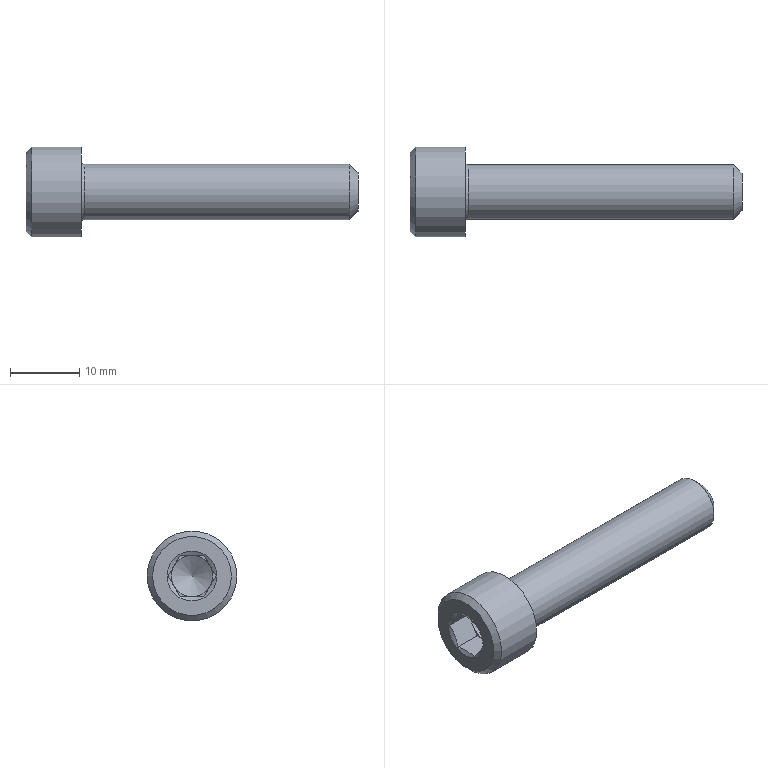Part | STEP file | Винт М8-6gx40 ГОСТ 11738-84 | 1 solid | 23 faces | box 48 x 13 x 13 mm | volume 2873 mm3 | plane 15 | cone 4 | cylinder 3 | torus 1 | commonest cylinder face diameters 6 x1 8 x1 13 x1
STEP:
#1=CARTESIAN_POINT('',(-8.,5.7,0.));
#2=VERTEX_POINT('',#1);
#3=CARTESIAN_POINT('',(-8.,0.,0.));
#4=DIRECTION('',(1.,0.,0.));
#5=DIRECTION('',(0.,1.,0.));
#6=AXIS2_PLACEMENT_3D('',#3,#4,#5);
#7=CIRCLE('',#6,5.7);
#8=EDGE_CURVE('',#2,#2,#7,.T.);
#9=ORIENTED_EDGE('',*,*,#8,.F.);
#10=EDGE_LOOP('',(#9));
#11=FACE_BOUND('',#10,.T.);
#12=CARTESIAN_POINT('',(-8.,3.6,0.));
#13=VERTEX_POINT('',#12);
#14=CARTESIAN_POINT('',(-8.,0.,0.));
#15=DIRECTION('',(1.,0.,0.));
#16=DIRECTION('',(0.,1.,0.));
#17=AXIS2_PLACEMENT_3D('',#14,#15,#16);
#18=CIRCLE('',#17,3.6);
#19=EDGE_CURVE('',#13,#13,#18,.T.);
#20=ORIENTED_EDGE('',*,*,#19,.T.);
#21=EDGE_LOOP('',(#20));
#22=FACE_BOUND('',#21,.T.);
#23=CARTESIAN_POINT('',(-8.,0.,0.));
#24=DIRECTION('',(-1.,0.,0.));
#25=DIRECTION('',(0.,1.,0.));
#26=AXIS2_PLACEMENT_3D('',#23,#24,#25);
#27=PLANE('',#26);
#28=ADVANCED_FACE('',(#11,#22),#27,.T.);
#29=CARTESIAN_POINT('',(-7.922,1.732,-3.));
#30=VERTEX_POINT('',#29);
#31=CARTESIAN_POINT('',(-7.922,-1.732,-3.));
#32=VERTEX_POINT('',#31);
#33=CARTESIAN_POINT('',(-7.922,1.732,-3.));
#34=CARTESIAN_POINT('',(-7.911,1.695,-3.));
#35=CARTESIAN_POINT('',(-7.891,1.625,-3.));
#36=CARTESIAN_POINT('',(-7.871,1.55,-3.));
#37=CARTESIAN_POINT('',(-7.851,1.474,-3.));
#38=CARTESIAN_POINT('',(-7.831,1.391,-3.));
#39=CARTESIAN_POINT('',(-7.803,1.276,-3.));
#40=CARTESIAN_POINT('',(-7.779,1.162,-3.));
#41=CARTESIAN_POINT('',(-7.76,1.068,-3.));
#42=CARTESIAN_POINT('',(-7.736,0.9374,-3.));
#43=CARTESIAN_POINT('',(-7.712,0.7953,-3.));
#44=CARTESIAN_POINT('',(-7.692,0.6398,-3.));
#45=CARTESIAN_POINT('',(-7.676,0.4906,-3.));
#46=CARTESIAN_POINT('',(-7.667,0.3765,-3.));
#47=CARTESIAN_POINT('',(-7.659,0.2523,-3.));
#48=CARTESIAN_POINT('',(-7.655,0.1456,-3.));
#49=CARTESIAN_POINT('',(-7.654,0.04767,-3.));
#50=CARTESIAN_POINT('',(-7.654,-0.05476,-3.));
#51=CARTESIAN_POINT('',(-7.655,-0.115,-3.));
#52=CARTESIAN_POINT('',(-7.658,-0.2282,-3.));
#53=CARTESIAN_POINT('',(-7.665,-0.3516,-3.));
#54=CARTESIAN_POINT('',(-7.676,-0.494,-3.));
#55=CARTESIAN_POINT('',(-7.689,-0.6078,-3.));
#56=CARTESIAN_POINT('',(-7.702,-0.7201,-3.));
#57=CARTESIAN_POINT('',(-7.719,-0.8365,-3.));
#58=CARTESIAN_POINT('',(-7.737,-0.9456,-3.));
#59=CARTESIAN_POINT('',(-7.756,-1.051,-3.));
#60=CARTESIAN_POINT('',(-7.781,-1.173,-3.));
#61=CARTESIAN_POINT('',(-7.808,-1.297,-3.));
#62=CARTESIAN_POINT('',(-7.831,-1.393,-3.));
#63=CARTESIAN_POINT('',(-7.854,-1.486,-3.));
#64=CARTESIAN_POINT('',(-7.882,-1.59,-3.));
#65=CARTESIAN_POINT('',(-7.906,-1.679,-3.));
#66=CARTESIAN_POINT('',(-7.919,-1.723,-3.));
#67=CARTESIAN_POINT('',(-7.922,-1.732,-3.));
#68=B_SPLINE_CURVE_WITH_KNOTS('',3,(#33,#34,#35,#36,#37,#38,#39,#40,#41,#42,#43,#44,#45,#46,#47,#48,#49,#50,#51,#52,#53,#54,#55,#56,#57,#58,#59,#60,#61,#62,#63,#64,#65,#66,#67),.UNSPECIFIED.,.F.,.F.,(4,1,1,1,1,1,1,1,1,1,1,1,1,1,1,1,1,1,1,1,1,1,1,1,1,1,1,1,1,1,1,1,4),(0.,0.03325,0.06137,0.06664,0.1002,0.134,0.1679,0.1994,0.2162,0.2809,0.3222,0.3499,0.4089,0.4198,0.456,0.5,0.5033,0.5434,0.5514,0.5999,0.6487,0.6732,0.6976,0.7453,0.7735,0.7919,0.8363,0.8796,0.9003,0.9208,0.9609,0.9923,1.),.UNSPECIFIED.);
#69=EDGE_CURVE('',#30,#32,#68,.T.);
#70=ORIENTED_EDGE('',*,*,#69,.T.);
#71=CARTESIAN_POINT('',(-4.,-1.732,-3.));
#72=VERTEX_POINT('',#71);
#73=CARTESIAN_POINT('',(-4.,-1.732,-3.));
#74=DIRECTION('',(-1.,0.,0.));
#75=VECTOR('',#74,1.);
#76=LINE('',#73,#75);
#77=EDGE_CURVE('',#72,#32,#76,.T.);
#78=ORIENTED_EDGE('',*,*,#77,.F.);
#79=CARTESIAN_POINT('',(-4.,0.,-3.));
#80=VERTEX_POINT('',#79);
#81=CARTESIAN_POINT('',(-4.,0.,-3.));
#82=DIRECTION('',(0.,-1.,0.));
#83=VECTOR('',#82,1.);
#84=LINE('',#81,#83);
#85=EDGE_CURVE('',#80,#72,#84,.T.);
#86=ORIENTED_EDGE('',*,*,#85,.F.);
#87=CARTESIAN_POINT('',(-4.,1.732,-3.));
#88=VERTEX_POINT('',#87);
#89=CARTESIAN_POINT('',(-4.,1.732,-3.));
#90=DIRECTION('',(0.,-1.,0.));
#91=VECTOR('',#90,1.);
#92=LINE('',#89,#91);
#93=EDGE_CURVE('',#88,#80,#92,.T.);
#94=ORIENTED_EDGE('',*,*,#93,.F.);
#95=CARTESIAN_POINT('',(-4.,1.732,-3.));
#96=DIRECTION('',(-1.,0.,0.));
#97=VECTOR('',#96,1.);
#98=LINE('',#95,#97);
#99=EDGE_CURVE('',#88,#30,#98,.T.);
#100=ORIENTED_EDGE('',*,*,#99,.T.);
#101=EDGE_LOOP('',(#70,#78,#86,#94,#100));
#102=FACE_BOUND('',#101,.T.);
#103=CARTESIAN_POINT('',(-4.,1.732,-3.));
#104=DIRECTION('',(0.,0.,-1.));
#105=DIRECTION('',(0.,-1.,0.));
#106=AXIS2_PLACEMENT_3D('',#103,#104,#105);
#107=PLANE('',#106);
#108=ADVANCED_FACE('',(#102),#107,.F.);
#109=CARTESIAN_POINT('',(-7.922,-3.464,0.));
#110=VERTEX_POINT('',#109);
#111=CARTESIAN_POINT('',(-7.922,-1.732,-3.));
#112=CARTESIAN_POINT('',(-7.911,-1.751,-2.968));
#113=CARTESIAN_POINT('',(-7.89,-1.788,-2.902));
#114=CARTESIAN_POINT('',(-7.859,-1.845,-2.804));
#115=CARTESIAN_POINT('',(-7.831,-1.902,-2.705));
#116=CARTESIAN_POINT('',(-7.803,-1.96,-2.605));
#117=CARTESIAN_POINT('',(-7.775,-2.027,-2.49));
#118=CARTESIAN_POINT('',(-7.741,-2.111,-2.343));
#119=CARTESIAN_POINT('',(-7.707,-2.216,-2.161));
#120=CARTESIAN_POINT('',(-7.68,-2.329,-1.967));
#121=CARTESIAN_POINT('',(-7.663,-2.431,-1.789));
#122=CARTESIAN_POINT('',(-7.655,-2.519,-1.637));
#123=CARTESIAN_POINT('',(-7.654,-2.574,-1.541));
#124=CARTESIAN_POINT('',(-7.654,-2.63,-1.444));
#125=CARTESIAN_POINT('',(-7.656,-2.689,-1.343));
#126=CARTESIAN_POINT('',(-7.665,-2.774,-1.196));
#127=CARTESIAN_POINT('',(-7.679,-2.859,-1.048));
#128=CARTESIAN_POINT('',(-7.698,-2.944,-0.901));
#129=CARTESIAN_POINT('',(-7.722,-3.027,-0.7571));
#130=CARTESIAN_POINT('',(-7.75,-3.107,-0.6183));
#131=CARTESIAN_POINT('',(-7.781,-3.184,-0.4844));
#132=CARTESIAN_POINT('',(-7.813,-3.258,-0.3566));
#133=CARTESIAN_POINT('',(-7.848,-3.329,-0.2336));
#134=CARTESIAN_POINT('',(-7.884,-3.397,-0.1154));
#135=CARTESIAN_POINT('',(-7.909,-3.442,-0.03806));
#136=CARTESIAN_POINT('',(-7.922,-3.464,-0.000000001));
#137=B_SPLINE_CURVE_WITH_KNOTS('',3,(#111,#112,#113,#114,#115,#116,#117,#118,#119,#120,#121,#122,#123,#124,#125,#126,#127,#128,#129,#130,#131,#132,#133,#134,#135,#136),.UNSPECIFIED.,.F.,.F.,(4,1,1,1,1,1,1,1,1,1,1,1,1,1,1,1,1,1,1,1,1,1,1,4),(0.,0.03325,0.06664,0.1002,0.134,0.1679,0.2162,0.2809,0.3499,0.4089,0.456,0.5,0.5033,0.5514,0.5999,0.6487,0.6976,0.7453,0.7919,0.8363,0.8796,0.9208,0.9609,1.),.UNSPECIFIED.);
#138=EDGE_CURVE('',#32,#110,#137,.T.);
#139=ORIENTED_EDGE('',*,*,#138,.T.);
#140=CARTESIAN_POINT('',(-4.,-3.464,0.));
#141=VERTEX_POINT('',#140);
#142=CARTESIAN_POINT('',(-4.,-3.464,0.));
#143=DIRECTION('',(-1.,0.,0.));
#144=VECTOR('',#143,1.);
#145=LINE('',#142,#144);
#146=EDGE_CURVE('',#141,#110,#145,.T.);
#147=ORIENTED_EDGE('',*,*,#146,.F.);
#148=CARTESIAN_POINT('',(-4.,-2.598,-1.5));
#149=VERTEX_POINT('',#148);
#150=CARTESIAN_POINT('',(-4.,-2.598,-1.5));
#151=DIRECTION('',(0.,-0.5,0.866));
#152=VECTOR('',#151,1.);
#153=LINE('',#150,#152);
#154=EDGE_CURVE('',#149,#141,#153,.T.);
#155=ORIENTED_EDGE('',*,*,#154,.F.);
#156=CARTESIAN_POINT('',(-4.,-1.732,-3.));
#157=DIRECTION('',(0.,-0.5,0.866));
#158=VECTOR('',#157,1.);
#159=LINE('',#156,#158);
#160=EDGE_CURVE('',#72,#149,#159,.T.);
#161=ORIENTED_EDGE('',*,*,#160,.F.);
#162=ORIENTED_EDGE('',*,*,#77,.T.);
#163=EDGE_LOOP('',(#139,#147,#155,#161,#162));
#164=FACE_BOUND('',#163,.T.);
#165=CARTESIAN_POINT('',(-4.,-1.732,-3.));
#166=DIRECTION('',(0.,-0.866,-0.5));
#167=DIRECTION('',(0.,-0.5,0.866));
#168=AXIS2_PLACEMENT_3D('',#165,#166,#167);
#169=PLANE('',#168);
#170=ADVANCED_FACE('',(#164),#169,.F.);
#171=CARTESIAN_POINT('',(-7.922,-1.732,3.));
#172=VERTEX_POINT('',#171);
#173=CARTESIAN_POINT('',(-7.922,-3.464,0.));
#174=CARTESIAN_POINT('',(-7.911,-3.445,0.03241));
#175=CARTESIAN_POINT('',(-7.89,-3.408,0.09751));
#176=CARTESIAN_POINT('',(-7.859,-3.351,0.1958));
#177=CARTESIAN_POINT('',(-7.831,-3.294,0.295));
#178=CARTESIAN_POINT('',(-7.803,-3.236,0.3951));
#179=CARTESIAN_POINT('',(-7.775,-3.17,0.5102));
#180=CARTESIAN_POINT('',(-7.741,-3.085,0.6567));
#181=CARTESIAN_POINT('',(-7.707,-2.98,0.839));
#182=CARTESIAN_POINT('',(-7.68,-2.867,1.033));
#183=CARTESIAN_POINT('',(-7.663,-2.765,1.211));
#184=CARTESIAN_POINT('',(-7.655,-2.677,1.363));
#185=CARTESIAN_POINT('',(-7.654,-2.622,1.459));
#186=CARTESIAN_POINT('',(-7.654,-2.566,1.556));
#187=CARTESIAN_POINT('',(-7.656,-2.507,1.657));
#188=CARTESIAN_POINT('',(-7.665,-2.422,1.804));
#189=CARTESIAN_POINT('',(-7.679,-2.337,1.952));
#190=CARTESIAN_POINT('',(-7.698,-2.252,2.099));
#191=CARTESIAN_POINT('',(-7.722,-2.169,2.243));
#192=CARTESIAN_POINT('',(-7.75,-2.089,2.382));
#193=CARTESIAN_POINT('',(-7.781,-2.012,2.516));
#194=CARTESIAN_POINT('',(-7.813,-1.938,2.643));
#195=CARTESIAN_POINT('',(-7.848,-1.867,2.766));
#196=CARTESIAN_POINT('',(-7.884,-1.799,2.885));
#197=CARTESIAN_POINT('',(-7.909,-1.754,2.962));
#198=CARTESIAN_POINT('',(-7.922,-1.732,3.));
#199=B_SPLINE_CURVE_WITH_KNOTS('',3,(#173,#174,#175,#176,#177,#178,#179,#180,#181,#182,#183,#184,#185,#186,#187,#188,#189,#190,#191,#192,#193,#194,#195,#196,#197,#198),.UNSPECIFIED.,.F.,.F.,(4,1,1,1,1,1,1,1,1,1,1,1,1,1,1,1,1,1,1,1,1,1,1,4),(0.,0.03325,0.06664,0.1002,0.134,0.1679,0.2162,0.2809,0.3499,0.4089,0.456,0.5,0.5033,0.5514,0.5999,0.6487,0.6976,0.7453,0.7919,0.8363,0.8796,0.9208,0.9609,1.),.UNSPECIFIED.);
#200=EDGE_CURVE('',#110,#172,#199,.T.);
#201=ORIENTED_EDGE('',*,*,#200,.T.);
#202=CARTESIAN_POINT('',(-4.,-1.732,3.));
#203=VERTEX_POINT('',#202);
#204=CARTESIAN_POINT('',(-4.,-1.732,3.));
#205=DIRECTION('',(-1.,0.,0.));
#206=VECTOR('',#205,1.);
#207=LINE('',#204,#206);
#208=EDGE_CURVE('',#203,#172,#207,.T.);
#209=ORIENTED_EDGE('',*,*,#208,.F.);
#210=CARTESIAN_POINT('',(-4.,-2.598,1.5));
#211=VERTEX_POINT('',#210);
#212=CARTESIAN_POINT('',(-4.,-2.598,1.5));
#213=DIRECTION('',(0.,0.5,0.866));
#214=VECTOR('',#213,1.);
#215=LINE('',#212,#214);
#216=EDGE_CURVE('',#211,#203,#215,.T.);
#217=ORIENTED_EDGE('',*,*,#216,.F.);
#218=CARTESIAN_POINT('',(-4.,-3.464,0.));
#219=DIRECTION('',(0.,0.5,0.866));
#220=VECTOR('',#219,1.);
#221=LINE('',#218,#220);
#222=EDGE_CURVE('',#141,#211,#221,.T.);
#223=ORIENTED_EDGE('',*,*,#222,.F.);
#224=ORIENTED_EDGE('',*,*,#146,.T.);
#225=EDGE_LOOP('',(#201,#209,#217,#223,#224));
#226=FACE_BOUND('',#225,.T.);
#227=CARTESIAN_POINT('',(-4.,-3.464,0.));
#228=DIRECTION('',(0.,-0.866,0.5));
#229=DIRECTION('',(0.,0.5,0.866));
#230=AXIS2_PLACEMENT_3D('',#227,#228,#229);
#231=PLANE('',#230);
#232=ADVANCED_FACE('',(#226),#231,.F.);
#233=CARTESIAN_POINT('',(-7.922,1.732,3.));
#234=VERTEX_POINT('',#233);
#235=CARTESIAN_POINT('',(-7.922,-1.732,3.));
#236=CARTESIAN_POINT('',(-7.911,-1.695,3.));
#237=CARTESIAN_POINT('',(-7.891,-1.625,3.));
#238=CARTESIAN_POINT('',(-7.871,-1.55,3.));
#239=CARTESIAN_POINT('',(-7.851,-1.474,3.));
#240=CARTESIAN_POINT('',(-7.831,-1.391,3.));
#241=CARTESIAN_POINT('',(-7.803,-1.276,3.));
#242=CARTESIAN_POINT('',(-7.779,-1.162,3.));
#243=CARTESIAN_POINT('',(-7.76,-1.068,3.));
#244=CARTESIAN_POINT('',(-7.736,-0.9374,3.));
#245=CARTESIAN_POINT('',(-7.712,-0.7953,3.));
#246=CARTESIAN_POINT('',(-7.692,-0.6398,3.));
#247=CARTESIAN_POINT('',(-7.676,-0.4906,3.));
#248=CARTESIAN_POINT('',(-7.667,-0.3765,3.));
#249=CARTESIAN_POINT('',(-7.659,-0.2523,3.));
#250=CARTESIAN_POINT('',(-7.655,-0.1456,3.));
#251=CARTESIAN_POINT('',(-7.654,-0.04767,3.));
#252=CARTESIAN_POINT('',(-7.654,0.05476,3.));
#253=CARTESIAN_POINT('',(-7.655,0.115,3.));
#254=CARTESIAN_POINT('',(-7.658,0.2282,3.));
#255=CARTESIAN_POINT('',(-7.665,0.3516,3.));
#256=CARTESIAN_POINT('',(-7.676,0.494,3.));
#257=CARTESIAN_POINT('',(-7.689,0.6078,3.));
#258=CARTESIAN_POINT('',(-7.702,0.7201,3.));
#259=CARTESIAN_POINT('',(-7.719,0.8365,3.));
#260=CARTESIAN_POINT('',(-7.737,0.9456,3.));
#261=CARTESIAN_POINT('',(-7.756,1.051,3.));
#262=CARTESIAN_POINT('',(-7.781,1.173,3.));
#263=CARTESIAN_POINT('',(-7.808,1.297,3.));
#264=CARTESIAN_POINT('',(-7.831,1.393,3.));
#265=CARTESIAN_POINT('',(-7.854,1.486,3.));
#266=CARTESIAN_POINT('',(-7.882,1.59,3.));
#267=CARTESIAN_POINT('',(-7.906,1.679,3.));
#268=CARTESIAN_POINT('',(-7.919,1.723,3.));
#269=CARTESIAN_POINT('',(-7.922,1.732,3.));
#270=B_SPLINE_CURVE_WITH_KNOTS('',3,(#235,#236,#237,#238,#239,#240,#241,#242,#243,#244,#245,#246,#247,#248,#249,#250,#251,#252,#253,#254,#255,#256,#257,#258,#259,#260,#261,#262,#263,#264,#265,#266,#267,#268,#269),.UNSPECIFIED.,.F.,.F.,(4,1,1,1,1,1,1,1,1,1,1,1,1,1,1,1,1,1,1,1,1,1,1,1,1,1,1,1,1,1,1,1,4),(0.,0.03325,0.06137,0.06664,0.1002,0.134,0.1679,0.1994,0.2162,0.2809,0.3222,0.3499,0.4089,0.4198,0.456,0.5,0.5033,0.5434,0.5514,0.5999,0.6487,0.6732,0.6976,0.7453,0.7735,0.7919,0.8363,0.8796,0.9003,0.9208,0.9609,0.9923,1.),.UNSPECIFIED.);
#271=EDGE_CURVE('',#172,#234,#270,.T.);
#272=ORIENTED_EDGE('',*,*,#271,.T.);
#273=CARTESIAN_POINT('',(-4.,1.732,3.));
#274=VERTEX_POINT('',#273);
#275=CARTESIAN_POINT('',(-4.,1.732,3.));
#276=DIRECTION('',(-1.,0.,0.));
#277=VECTOR('',#276,1.);
#278=LINE('',#275,#277);
#279=EDGE_CURVE('',#274,#234,#278,.T.);
#280=ORIENTED_EDGE('',*,*,#279,.F.);
#281=CARTESIAN_POINT('',(-4.,0.,3.));
#282=VERTEX_POINT('',#281);
#283=CARTESIAN_POINT('',(-4.,0.,3.));
#284=DIRECTION('',(0.,1.,0.));
#285=VECTOR('',#284,1.);
#286=LINE('',#283,#285);
#287=EDGE_CURVE('',#282,#274,#286,.T.);
#288=ORIENTED_EDGE('',*,*,#287,.F.);
#289=CARTESIAN_POINT('',(-4.,-1.732,3.));
#290=DIRECTION('',(0.,1.,0.));
#291=VECTOR('',#290,1.);
#292=LINE('',#289,#291);
#293=EDGE_CURVE('',#203,#282,#292,.T.);
#294=ORIENTED_EDGE('',*,*,#293,.F.);
#295=ORIENTED_EDGE('',*,*,#208,.T.);
#296=EDGE_LOOP('',(#272,#280,#288,#294,#295));
#297=FACE_BOUND('',#296,.T.);
#298=CARTESIAN_POINT('',(-4.,-1.732,3.));
#299=DIRECTION('',(0.,0.,1.));
#300=DIRECTION('',(0.,1.,0.));
#301=AXIS2_PLACEMENT_3D('',#298,#299,#300);
#302=PLANE('',#301);
#303=ADVANCED_FACE('',(#297),#302,.F.);
#304=CARTESIAN_POINT('',(-7.922,3.464,0.));
#305=VERTEX_POINT('',#304);
#306=CARTESIAN_POINT('',(-7.922,3.464,0.));
#307=CARTESIAN_POINT('',(-7.911,3.445,-0.03242));
#308=CARTESIAN_POINT('',(-7.89,3.408,-0.09751));
#309=CARTESIAN_POINT('',(-7.859,3.351,-0.1958));
#310=CARTESIAN_POINT('',(-7.831,3.294,-0.295));
#311=CARTESIAN_POINT('',(-7.803,3.236,-0.3951));
#312=CARTESIAN_POINT('',(-7.775,3.17,-0.5102));
#313=CARTESIAN_POINT('',(-7.741,3.085,-0.6567));
#314=CARTESIAN_POINT('',(-7.707,2.98,-0.839));
#315=CARTESIAN_POINT('',(-7.68,2.867,-1.033));
#316=CARTESIAN_POINT('',(-7.663,2.765,-1.211));
#317=CARTESIAN_POINT('',(-7.655,2.677,-1.363));
#318=CARTESIAN_POINT('',(-7.654,2.622,-1.459));
#319=CARTESIAN_POINT('',(-7.654,2.566,-1.556));
#320=CARTESIAN_POINT('',(-7.656,2.507,-1.657));
#321=CARTESIAN_POINT('',(-7.665,2.422,-1.805));
#322=CARTESIAN_POINT('',(-7.679,2.337,-1.952));
#323=CARTESIAN_POINT('',(-7.698,2.252,-2.099));
#324=CARTESIAN_POINT('',(-7.722,2.169,-2.243));
#325=CARTESIAN_POINT('',(-7.75,2.089,-2.382));
#326=CARTESIAN_POINT('',(-7.781,2.012,-2.516));
#327=CARTESIAN_POINT('',(-7.813,1.938,-2.643));
#328=CARTESIAN_POINT('',(-7.848,1.867,-2.766));
#329=CARTESIAN_POINT('',(-7.884,1.799,-2.885));
#330=CARTESIAN_POINT('',(-7.909,1.754,-2.962));
#331=CARTESIAN_POINT('',(-7.922,1.732,-3.));
#332=B_SPLINE_CURVE_WITH_KNOTS('',3,(#306,#307,#308,#309,#310,#311,#312,#313,#314,#315,#316,#317,#318,#319,#320,#321,#322,#323,#324,#325,#326,#327,#328,#329,#330,#331),.UNSPECIFIED.,.F.,.F.,(4,1,1,1,1,1,1,1,1,1,1,1,1,1,1,1,1,1,1,1,1,1,1,4),(0.,0.03325,0.06664,0.1002,0.134,0.1679,0.2162,0.2809,0.3499,0.4089,0.456,0.5,0.5033,0.5514,0.5999,0.6487,0.6976,0.7453,0.7919,0.8363,0.8796,0.9208,0.9609,1.),.UNSPECIFIED.);
#333=EDGE_CURVE('',#305,#30,#332,.T.);
#334=ORIENTED_EDGE('',*,*,#333,.T.);
#335=ORIENTED_EDGE('',*,*,#99,.F.);
#336=CARTESIAN_POINT('',(-4.,2.598,-1.5));
#337=VERTEX_POINT('',#336);
#338=CARTESIAN_POINT('',(-4.,2.598,-1.5));
#339=DIRECTION('',(0.,-0.5,-0.866));
#340=VECTOR('',#339,1.);
#341=LINE('',#338,#340);
#342=EDGE_CURVE('',#337,#88,#341,.T.);
#343=ORIENTED_EDGE('',*,*,#342,.F.);
#344=CARTESIAN_POINT('',(-4.,3.464,0.));
#345=VERTEX_POINT('',#344);
#346=CARTESIAN_POINT('',(-4.,3.464,0.));
#347=DIRECTION('',(0.,-0.5,-0.866));
#348=VECTOR('',#347,1.);
#349=LINE('',#346,#348);
#350=EDGE_CURVE('',#345,#337,#349,.T.);
#351=ORIENTED_EDGE('',*,*,#350,.F.);
#352=CARTESIAN_POINT('',(-4.,3.464,0.));
#353=DIRECTION('',(-1.,0.,0.));
#354=VECTOR('',#353,1.);
#355=LINE('',#352,#354);
#356=EDGE_CURVE('',#345,#305,#355,.T.);
#357=ORIENTED_EDGE('',*,*,#356,.T.);
#358=EDGE_LOOP('',(#334,#335,#343,#351,#357));
#359=FACE_BOUND('',#358,.T.);
#360=CARTESIAN_POINT('',(-4.,3.464,0.));
#361=DIRECTION('',(0.,0.866,-0.5));
#362=DIRECTION('',(0.,-0.5,-0.866));
#363=AXIS2_PLACEMENT_3D('',#360,#361,#362);
#364=PLANE('',#363);
#365=ADVANCED_FACE('',(#359),#364,.F.);
#366=CARTESIAN_POINT('',(-7.922,1.732,3.));
#367=CARTESIAN_POINT('',(-7.911,1.751,2.968));
#368=CARTESIAN_POINT('',(-7.89,1.788,2.902));
#369=CARTESIAN_POINT('',(-7.859,1.845,2.804));
#370=CARTESIAN_POINT('',(-7.831,1.902,2.705));
#371=CARTESIAN_POINT('',(-7.803,1.96,2.605));
#372=CARTESIAN_POINT('',(-7.775,2.027,2.49));
#373=CARTESIAN_POINT('',(-7.741,2.111,2.343));
#374=CARTESIAN_POINT('',(-7.707,2.216,2.161));
#375=CARTESIAN_POINT('',(-7.68,2.329,1.967));
#376=CARTESIAN_POINT('',(-7.663,2.431,1.789));
#377=CARTESIAN_POINT('',(-7.655,2.519,1.637));
#378=CARTESIAN_POINT('',(-7.654,2.574,1.541));
#379=CARTESIAN_POINT('',(-7.654,2.63,1.444));
#380=CARTESIAN_POINT('',(-7.656,2.689,1.343));
#381=CARTESIAN_POINT('',(-7.665,2.774,1.195));
#382=CARTESIAN_POINT('',(-7.679,2.859,1.048));
#383=CARTESIAN_POINT('',(-7.698,2.944,0.9009));
#384=CARTESIAN_POINT('',(-7.722,3.027,0.7571));
#385=CARTESIAN_POINT('',(-7.75,3.107,0.6183));
#386=CARTESIAN_POINT('',(-7.781,3.184,0.4844));
#387=CARTESIAN_POINT('',(-7.813,3.258,0.3566));
#388=CARTESIAN_POINT('',(-7.848,3.329,0.2336));
#389=CARTESIAN_POINT('',(-7.884,3.397,0.1154));
#390=CARTESIAN_POINT('',(-7.909,3.442,0.03806));
#391=CARTESIAN_POINT('',(-7.922,3.464,0.));
#392=B_SPLINE_CURVE_WITH_KNOTS('',3,(#366,#367,#368,#369,#370,#371,#372,#373,#374,#375,#376,#377,#378,#379,#380,#381,#382,#383,#384,#385,#386,#387,#388,#389,#390,#391),.UNSPECIFIED.,.F.,.F.,(4,1,1,1,1,1,1,1,1,1,1,1,1,1,1,1,1,1,1,1,1,1,1,4),(0.,0.03325,0.06664,0.1002,0.134,0.1679,0.2162,0.2809,0.3499,0.4089,0.456,0.5,0.5033,0.5514,0.5999,0.6487,0.6976,0.7453,0.7919,0.8363,0.8796,0.9208,0.9609,1.),.UNSPECIFIED.);
#393=EDGE_CURVE('',#234,#305,#392,.T.);
#394=ORIENTED_EDGE('',*,*,#393,.T.);
#395=ORIENTED_EDGE('',*,*,#356,.F.);
#396=CARTESIAN_POINT('',(-4.,2.598,1.5));
#397=VERTEX_POINT('',#396);
#398=CARTESIAN_POINT('',(-4.,2.598,1.5));
#399=DIRECTION('',(0.,0.5,-0.866));
#400=VECTOR('',#399,1.);
#401=LINE('',#398,#400);
#402=EDGE_CURVE('',#397,#345,#401,.T.);
#403=ORIENTED_EDGE('',*,*,#402,.F.);
#404=CARTESIAN_POINT('',(-4.,1.732,3.));
#405=DIRECTION('',(0.,0.5,-0.866));
#406=VECTOR('',#405,1.);
#407=LINE('',#404,#406);
#408=EDGE_CURVE('',#274,#397,#407,.T.);
#409=ORIENTED_EDGE('',*,*,#408,.F.);
#410=ORIENTED_EDGE('',*,*,#279,.T.);
#411=EDGE_LOOP('',(#394,#395,#403,#409,#410));
#412=FACE_BOUND('',#411,.T.);
#413=CARTESIAN_POINT('',(-4.,1.732,3.));
#414=DIRECTION('',(0.,0.866,0.5));
#415=DIRECTION('',(0.,0.5,-0.866));
#416=AXIS2_PLACEMENT_3D('',#413,#414,#415);
#417=PLANE('',#416);
#418=ADVANCED_FACE('',(#412),#417,.F.);
#419=ORIENTED_EDGE('',*,*,#393,.F.);
#420=ORIENTED_EDGE('',*,*,#271,.F.);
#421=ORIENTED_EDGE('',*,*,#200,.F.);
#422=ORIENTED_EDGE('',*,*,#138,.F.);
#423=ORIENTED_EDGE('',*,*,#69,.F.);
#424=ORIENTED_EDGE('',*,*,#333,.F.);
#425=EDGE_LOOP('',(#419,#420,#421,#422,#423,#424));
#426=FACE_BOUND('',#425,.T.);
#427=ORIENTED_EDGE('',*,*,#19,.F.);
#428=EDGE_LOOP('',(#427));
#429=FACE_OUTER_BOUND('',#428,.T.);
#430=CARTESIAN_POINT('',(-7.827,0.,0.));
#431=DIRECTION('',(-1.,0.,0.));
#432=DIRECTION('',(0.,-1.,0.));
#433=AXIS2_PLACEMENT_3D('',#430,#431,#432);
#434=CONICAL_SURFACE('',#433,3.3,1.047);
#435=ADVANCED_FACE('',(#426,#429),#434,.F.);
#436=CARTESIAN_POINT('',(-7.2,6.5,0.));
#437=VERTEX_POINT('',#436);
#438=CARTESIAN_POINT('',(-7.2,0.,0.));
#439=DIRECTION('',(1.,0.,0.));
#440=DIRECTION('',(0.,1.,0.));
#441=AXIS2_PLACEMENT_3D('',#438,#439,#440);
#442=CIRCLE('',#441,6.5);
#443=EDGE_CURVE('',#437,#437,#442,.T.);
#444=ORIENTED_EDGE('',*,*,#443,.F.);
#445=EDGE_LOOP('',(#444));
#446=FACE_OUTER_BOUND('',#445,.T.);
#447=ORIENTED_EDGE('',*,*,#8,.T.);
#448=EDGE_LOOP('',(#447));
#449=FACE_OUTER_BOUND('',#448,.T.);
#450=CARTESIAN_POINT('',(-7.6,0.,0.));
#451=DIRECTION('',(1.,0.,0.));
#452=DIRECTION('',(0.,1.,0.));
#453=AXIS2_PLACEMENT_3D('',#450,#451,#452);
#454=CONICAL_SURFACE('',#453,6.1,0.7854);
#455=ADVANCED_FACE('',(#446,#449),#454,.T.);
#456=CARTESIAN_POINT('',(-4.,0.,0.));
#457=DIRECTION('',(1.,0.,0.));
#458=DIRECTION('',(0.,-0.866,-0.5));
#459=AXIS2_PLACEMENT_3D('',#456,#457,#458);
#460=CIRCLE('',#459,3.);
#461=EDGE_CURVE('',#149,#80,#460,.T.);
#462=ORIENTED_EDGE('',*,*,#461,.T.);
#463=ORIENTED_EDGE('',*,*,#85,.T.);
#464=ORIENTED_EDGE('',*,*,#160,.T.);
#465=EDGE_LOOP('',(#462,#463,#464));
#466=FACE_BOUND('',#465,.T.);
#467=CARTESIAN_POINT('',(-4.,0.,0.));
#468=DIRECTION('',(-1.,0.,0.));
#469=DIRECTION('',(0.,0.,-1.));
#470=AXIS2_PLACEMENT_3D('',#467,#468,#469);
#471=PLANE('',#470);
#472=ADVANCED_FACE('',(#466),#471,.T.);
#473=CARTESIAN_POINT('',(-4.,0.,0.));
#474=DIRECTION('',(1.,0.,0.));
#475=DIRECTION('',(0.,0.,-1.));
#476=AXIS2_PLACEMENT_3D('',#473,#474,#475);
#477=CIRCLE('',#476,3.);
#478=EDGE_CURVE('',#80,#337,#477,.T.);
#479=ORIENTED_EDGE('',*,*,#478,.T.);
#480=ORIENTED_EDGE('',*,*,#342,.T.);
#481=ORIENTED_EDGE('',*,*,#93,.T.);
#482=EDGE_LOOP('',(#479,#480,#481));
#483=FACE_BOUND('',#482,.T.);
#484=CARTESIAN_POINT('',(-4.,0.,0.));
#485=DIRECTION('',(-1.,0.,0.));
#486=DIRECTION('',(0.,0.,-1.));
#487=AXIS2_PLACEMENT_3D('',#484,#485,#486);
#488=PLANE('',#487);
#489=ADVANCED_FACE('',(#483),#488,.T.);
#490=CARTESIAN_POINT('',(-4.,0.,0.));
#491=DIRECTION('',(1.,0.,0.));
#492=DIRECTION('',(0.,-0.866,0.5));
#493=AXIS2_PLACEMENT_3D('',#490,#491,#492);
#494=CIRCLE('',#493,3.);
#495=EDGE_CURVE('',#211,#149,#494,.T.);
#496=ORIENTED_EDGE('',*,*,#495,.T.);
#497=ORIENTED_EDGE('',*,*,#154,.T.);
#498=ORIENTED_EDGE('',*,*,#222,.T.);
#499=EDGE_LOOP('',(#496,#497,#498));
#500=FACE_BOUND('',#499,.T.);
#501=CARTESIAN_POINT('',(-4.,0.,0.));
#502=DIRECTION('',(-1.,0.,0.));
#503=DIRECTION('',(0.,0.,-1.));
#504=AXIS2_PLACEMENT_3D('',#501,#502,#503);
#505=PLANE('',#504);
#506=ADVANCED_FACE('',(#500),#505,.T.);
#507=CARTESIAN_POINT('',(-4.,0.,0.));
#508=DIRECTION('',(1.,0.,0.));
#509=DIRECTION('',(0.,0.,1.));
#510=AXIS2_PLACEMENT_3D('',#507,#508,#509);
#511=CIRCLE('',#510,3.);
#512=EDGE_CURVE('',#282,#211,#511,.T.);
#513=ORIENTED_EDGE('',*,*,#512,.T.);
#514=ORIENTED_EDGE('',*,*,#216,.T.);
#515=ORIENTED_EDGE('',*,*,#293,.T.);
#516=EDGE_LOOP('',(#513,#514,#515));
#517=FACE_BOUND('',#516,.T.);
#518=CARTESIAN_POINT('',(-4.,0.,0.));
#519=DIRECTION('',(-1.,0.,0.));
#520=DIRECTION('',(0.,0.,-1.));
#521=AXIS2_PLACEMENT_3D('',#518,#519,#520);
#522=PLANE('',#521);
#523=ADVANCED_FACE('',(#517),#522,.T.);
#524=CARTESIAN_POINT('',(-4.,0.,0.));
#525=DIRECTION('',(1.,0.,0.));
#526=DIRECTION('',(0.,0.866,0.5));
#527=AXIS2_PLACEMENT_3D('',#524,#525,#526);
#528=CIRCLE('',#527,3.);
#529=EDGE_CURVE('',#397,#282,#528,.T.);
#530=ORIENTED_EDGE('',*,*,#529,.T.);
#531=ORIENTED_EDGE('',*,*,#287,.T.);
#532=ORIENTED_EDGE('',*,*,#408,.T.);
#533=EDGE_LOOP('',(#530,#531,#532));
#534=FACE_BOUND('',#533,.T.);
#535=CARTESIAN_POINT('',(-4.,0.,0.));
#536=DIRECTION('',(-1.,0.,0.));
#537=DIRECTION('',(0.,0.,-1.));
#538=AXIS2_PLACEMENT_3D('',#535,#536,#537);
#539=PLANE('',#538);
#540=ADVANCED_FACE('',(#534),#539,.T.);
#541=CARTESIAN_POINT('',(-4.,3.,0.));
#542=VERTEX_POINT('',#541);
#543=CARTESIAN_POINT('',(-4.,0.,0.));
#544=DIRECTION('',(1.,0.,0.));
#545=DIRECTION('',(0.,1.,0.));
#546=AXIS2_PLACEMENT_3D('',#543,#544,#545);
#547=CIRCLE('',#546,3.);
#548=EDGE_CURVE('',#542,#397,#547,.T.);
#549=ORIENTED_EDGE('',*,*,#548,.T.);
#550=ORIENTED_EDGE('',*,*,#402,.T.);
#551=ORIENTED_EDGE('',*,*,#350,.T.);
#552=CARTESIAN_POINT('',(-4.,0.,0.));
#553=DIRECTION('',(1.,0.,0.));
#554=DIRECTION('',(0.,0.866,-0.5));
#555=AXIS2_PLACEMENT_3D('',#552,#553,#554);
#556=CIRCLE('',#555,3.);
#557=EDGE_CURVE('',#337,#542,#556,.T.);
#558=ORIENTED_EDGE('',*,*,#557,.T.);
#559=EDGE_LOOP('',(#549,#550,#551,#558));
#560=FACE_BOUND('',#559,.T.);
#561=CARTESIAN_POINT('',(-4.,0.,0.));
#562=DIRECTION('',(-1.,0.,0.));
#563=DIRECTION('',(0.,0.,-1.));
#564=AXIS2_PLACEMENT_3D('',#561,#562,#563);
#565=PLANE('',#564);
#566=ADVANCED_FACE('',(#560),#565,.T.);
#567=CARTESIAN_POINT('',(0.,6.5,0.));
#568=VERTEX_POINT('',#567);
#569=CARTESIAN_POINT('',(0.,0.,0.));
#570=DIRECTION('',(1.,0.,0.));
#571=DIRECTION('',(0.,1.,0.));
#572=AXIS2_PLACEMENT_3D('',#569,#570,#571);
#573=CIRCLE('',#572,6.5);
#574=EDGE_CURVE('',#568,#568,#573,.T.);
#575=ORIENTED_EDGE('',*,*,#574,.F.);
#576=EDGE_LOOP('',(#575));
#577=FACE_OUTER_BOUND('',#576,.T.);
#578=ORIENTED_EDGE('',*,*,#443,.T.);
#579=EDGE_LOOP('',(#578));
#580=FACE_OUTER_BOUND('',#579,.T.);
#581=CARTESIAN_POINT('',(-8.,0.,0.));
#582=DIRECTION('',(1.,0.,0.));
#583=DIRECTION('',(0.,1.,0.));
#584=AXIS2_PLACEMENT_3D('',#581,#582,#583);
#585=CYLINDRICAL_SURFACE('',#584,6.5);
#586=ADVANCED_FACE('',(#577,#580),#585,.T.);
#587=CARTESIAN_POINT('',(-3.,3.,0.));
#588=VERTEX_POINT('',#587);
#589=CARTESIAN_POINT('',(-3.,0.,0.));
#590=DIRECTION('',(1.,0.,0.));
#591=DIRECTION('',(0.,1.,0.));
#592=AXIS2_PLACEMENT_3D('',#589,#590,#591);
#593=CIRCLE('',#592,3.);
#594=EDGE_CURVE('',#588,#588,#593,.T.);
#595=ORIENTED_EDGE('',*,*,#594,.T.);
#596=EDGE_LOOP('',(#595));
#597=FACE_OUTER_BOUND('',#596,.T.);
#598=ORIENTED_EDGE('',*,*,#557,.F.);
#599=ORIENTED_EDGE('',*,*,#478,.F.);
#600=ORIENTED_EDGE('',*,*,#461,.F.);
#601=ORIENTED_EDGE('',*,*,#495,.F.);
#602=ORIENTED_EDGE('',*,*,#512,.F.);
#603=ORIENTED_EDGE('',*,*,#529,.F.);
#604=ORIENTED_EDGE('',*,*,#548,.F.);
#605=EDGE_LOOP('',(#598,#599,#600,#601,#602,#603,#604));
#606=FACE_BOUND('',#605,.T.);
#607=CARTESIAN_POINT('',(-8.,0.,0.));
#608=DIRECTION('',(1.,0.,0.));
#609=DIRECTION('',(0.,1.,0.));
#610=AXIS2_PLACEMENT_3D('',#607,#608,#609);
#611=CYLINDRICAL_SURFACE('',#610,3.);
#612=ADVANCED_FACE('',(#597,#606),#611,.F.);
#613=ORIENTED_EDGE('',*,*,#574,.T.);
#614=EDGE_LOOP('',(#613));
#615=FACE_BOUND('',#614,.T.);
#616=CARTESIAN_POINT('',(0.,0.,-4.4));
#617=VERTEX_POINT('',#616);
#618=CARTESIAN_POINT('',(0.,0.,0.));
#619=DIRECTION('',(-1.,0.,0.));
#620=DIRECTION('',(0.,0.,-1.));
#621=AXIS2_PLACEMENT_3D('',#618,#619,#620);
#622=CIRCLE('',#621,4.4);
#623=EDGE_CURVE('',#617,#617,#622,.T.);
#624=ORIENTED_EDGE('',*,*,#623,.T.);
#625=EDGE_LOOP('',(#624));
#626=FACE_BOUND('',#625,.T.);
#627=CARTESIAN_POINT('',(0.,0.,0.));
#628=DIRECTION('',(1.,0.,0.));
#629=DIRECTION('',(0.,1.,0.));
#630=AXIS2_PLACEMENT_3D('',#627,#628,#629);
#631=PLANE('',#630);
#632=ADVANCED_FACE('',(#615,#626),#631,.T.);
#633=ORIENTED_EDGE('',*,*,#594,.F.);
#634=EDGE_LOOP('',(#633));
#635=FACE_OUTER_BOUND('',#634,.T.);
#636=CARTESIAN_POINT('',(-2.134,0.,0.));
#637=DIRECTION('',(-1.,0.,0.));
#638=DIRECTION('',(0.,-1.,0.));
#639=AXIS2_PLACEMENT_3D('',#636,#637,#638);
#640=CONICAL_SURFACE('',#639,1.5,1.047);
#641=ADVANCED_FACE('',(#635),#640,.F.);
#642=CARTESIAN_POINT('',(0.4,0.,-4.));
#643=VERTEX_POINT('',#642);
#644=CARTESIAN_POINT('',(0.4,0.,0.));
#645=DIRECTION('',(-1.,0.,0.));
#646=DIRECTION('',(0.,0.,-1.));
#647=AXIS2_PLACEMENT_3D('',#644,#645,#646);
#648=CIRCLE('',#647,4.);
#649=EDGE_CURVE('',#643,#643,#648,.T.);
#650=ORIENTED_EDGE('',*,*,#649,.T.);
#651=EDGE_LOOP('',(#650));
#652=FACE_OUTER_BOUND('',#651,.T.);
#653=ORIENTED_EDGE('',*,*,#623,.F.);
#654=EDGE_LOOP('',(#653));
#655=FACE_OUTER_BOUND('',#654,.T.);
#656=CARTESIAN_POINT('',(0.4,0.,0.));
#657=DIRECTION('',(-1.,0.,0.));
#658=DIRECTION('',(0.,0.,-1.));
#659=AXIS2_PLACEMENT_3D('',#656,#657,#658);
#660=TOROIDAL_SURFACE('',#659,4.4,0.4);
#661=ADVANCED_FACE('',(#652,#655),#660,.F.);
#662=CARTESIAN_POINT('',(38.75,0.,-4.));
#663=VERTEX_POINT('',#662);
#664=CARTESIAN_POINT('',(38.75,0.,0.));
#665=DIRECTION('',(-1.,0.,0.));
#666=DIRECTION('',(0.,0.,-1.));
#667=AXIS2_PLACEMENT_3D('',#664,#665,#666);
#668=CIRCLE('',#667,4.);
#669=EDGE_CURVE('',#663,#663,#668,.T.);
#670=ORIENTED_EDGE('',*,*,#669,.T.);
#671=EDGE_LOOP('',(#670));
#672=FACE_OUTER_BOUND('',#671,.T.);
#673=ORIENTED_EDGE('',*,*,#649,.F.);
#674=EDGE_LOOP('',(#673));
#675=FACE_OUTER_BOUND('',#674,.T.);
#676=CARTESIAN_POINT('',(40.,0.,0.));
#677=DIRECTION('',(-1.,0.,0.));
#678=DIRECTION('',(0.,0.,-1.));
#679=AXIS2_PLACEMENT_3D('',#676,#677,#678);
#680=CYLINDRICAL_SURFACE('',#679,4.);
#681=ADVANCED_FACE('',(#672,#675),#680,.T.);
#682=CARTESIAN_POINT('',(40.,0.,-2.75));
#683=VERTEX_POINT('',#682);
#684=CARTESIAN_POINT('',(40.,0.,0.));
#685=DIRECTION('',(-1.,0.,0.));
#686=DIRECTION('',(0.,0.,-1.));
#687=AXIS2_PLACEMENT_3D('',#684,#685,#686);
#688=CIRCLE('',#687,2.75);
#689=EDGE_CURVE('',#683,#683,#688,.T.);
#690=ORIENTED_EDGE('',*,*,#689,.F.);
#691=EDGE_LOOP('',(#690));
#692=FACE_BOUND('',#691,.T.);
#693=CARTESIAN_POINT('',(40.,0.,0.));
#694=DIRECTION('',(-1.,0.,0.));
#695=DIRECTION('',(0.,0.,-1.));
#696=AXIS2_PLACEMENT_3D('',#693,#694,#695);
#697=PLANE('',#696);
#698=ADVANCED_FACE('',(#692),#697,.F.);
#699=ORIENTED_EDGE('',*,*,#689,.T.);
#700=EDGE_LOOP('',(#699));
#701=FACE_OUTER_BOUND('',#700,.T.);
#702=ORIENTED_EDGE('',*,*,#669,.F.);
#703=EDGE_LOOP('',(#702));
#704=FACE_OUTER_BOUND('',#703,.T.);
#705=CARTESIAN_POINT('',(39.375,0.,0.));
#706=DIRECTION('',(-1.,0.,0.));
#707=DIRECTION('',(0.,0.,-1.));
#708=AXIS2_PLACEMENT_3D('',#705,#706,#707);
#709=CONICAL_SURFACE('',#708,3.375,0.7854);
#710=ADVANCED_FACE('',(#701,#704),#709,.T.);
#711=CLOSED_SHELL('',(#28,#108,#170,#232,#303,#365,#418,#435,#455,#472,#489,#506,#523,#540,#566,#586,#612,#632,#641,#661,#681,#698,#710));
#712=MANIFOLD_SOLID_BREP('',#711);
#713=(LENGTH_UNIT()NAMED_UNIT(*)SI_UNIT(.MILLI.,.METRE.));
#714=UNCERTAINTY_MEASURE_WITH_UNIT(LENGTH_MEASURE(0.00001),#713,'','');
#715=(NAMED_UNIT(*)PLANE_ANGLE_UNIT()SI_UNIT($,.RADIAN.));
#716=(NAMED_UNIT(*)SI_UNIT($,.STERADIAN.)SOLID_ANGLE_UNIT());
#717=(GEOMETRIC_REPRESENTATION_CONTEXT(3)GLOBAL_UNCERTAINTY_ASSIGNED_CONTEXT((#714))GLOBAL_UNIT_ASSIGNED_CONTEXT((#713,#715,#716))REPRESENTATION_CONTEXT('',''));
#718=ADVANCED_BREP_SHAPE_REPRESENTATION('',(#712),#717);